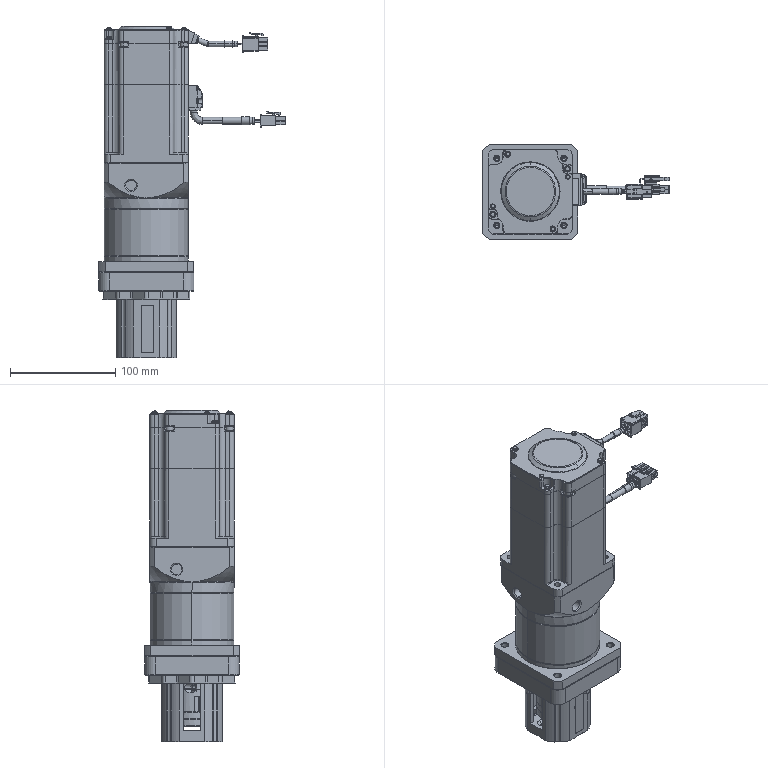Part | STEP file | Copy of 90 reducer-universal motor base^K50A-1H20-S(formula driven)-L300-motor left- | 14 solids | 1665 faces | box 176.65 x 90 x 314 mm | volume 1490817 mm3 | plane 761 | cylinder 605 | cone 184 | spline 70 | torus 45 | commonest cylinder face diameters 1 x82 8 x48 6 x37 2.6 x30 4.5 x24 0.5 x16